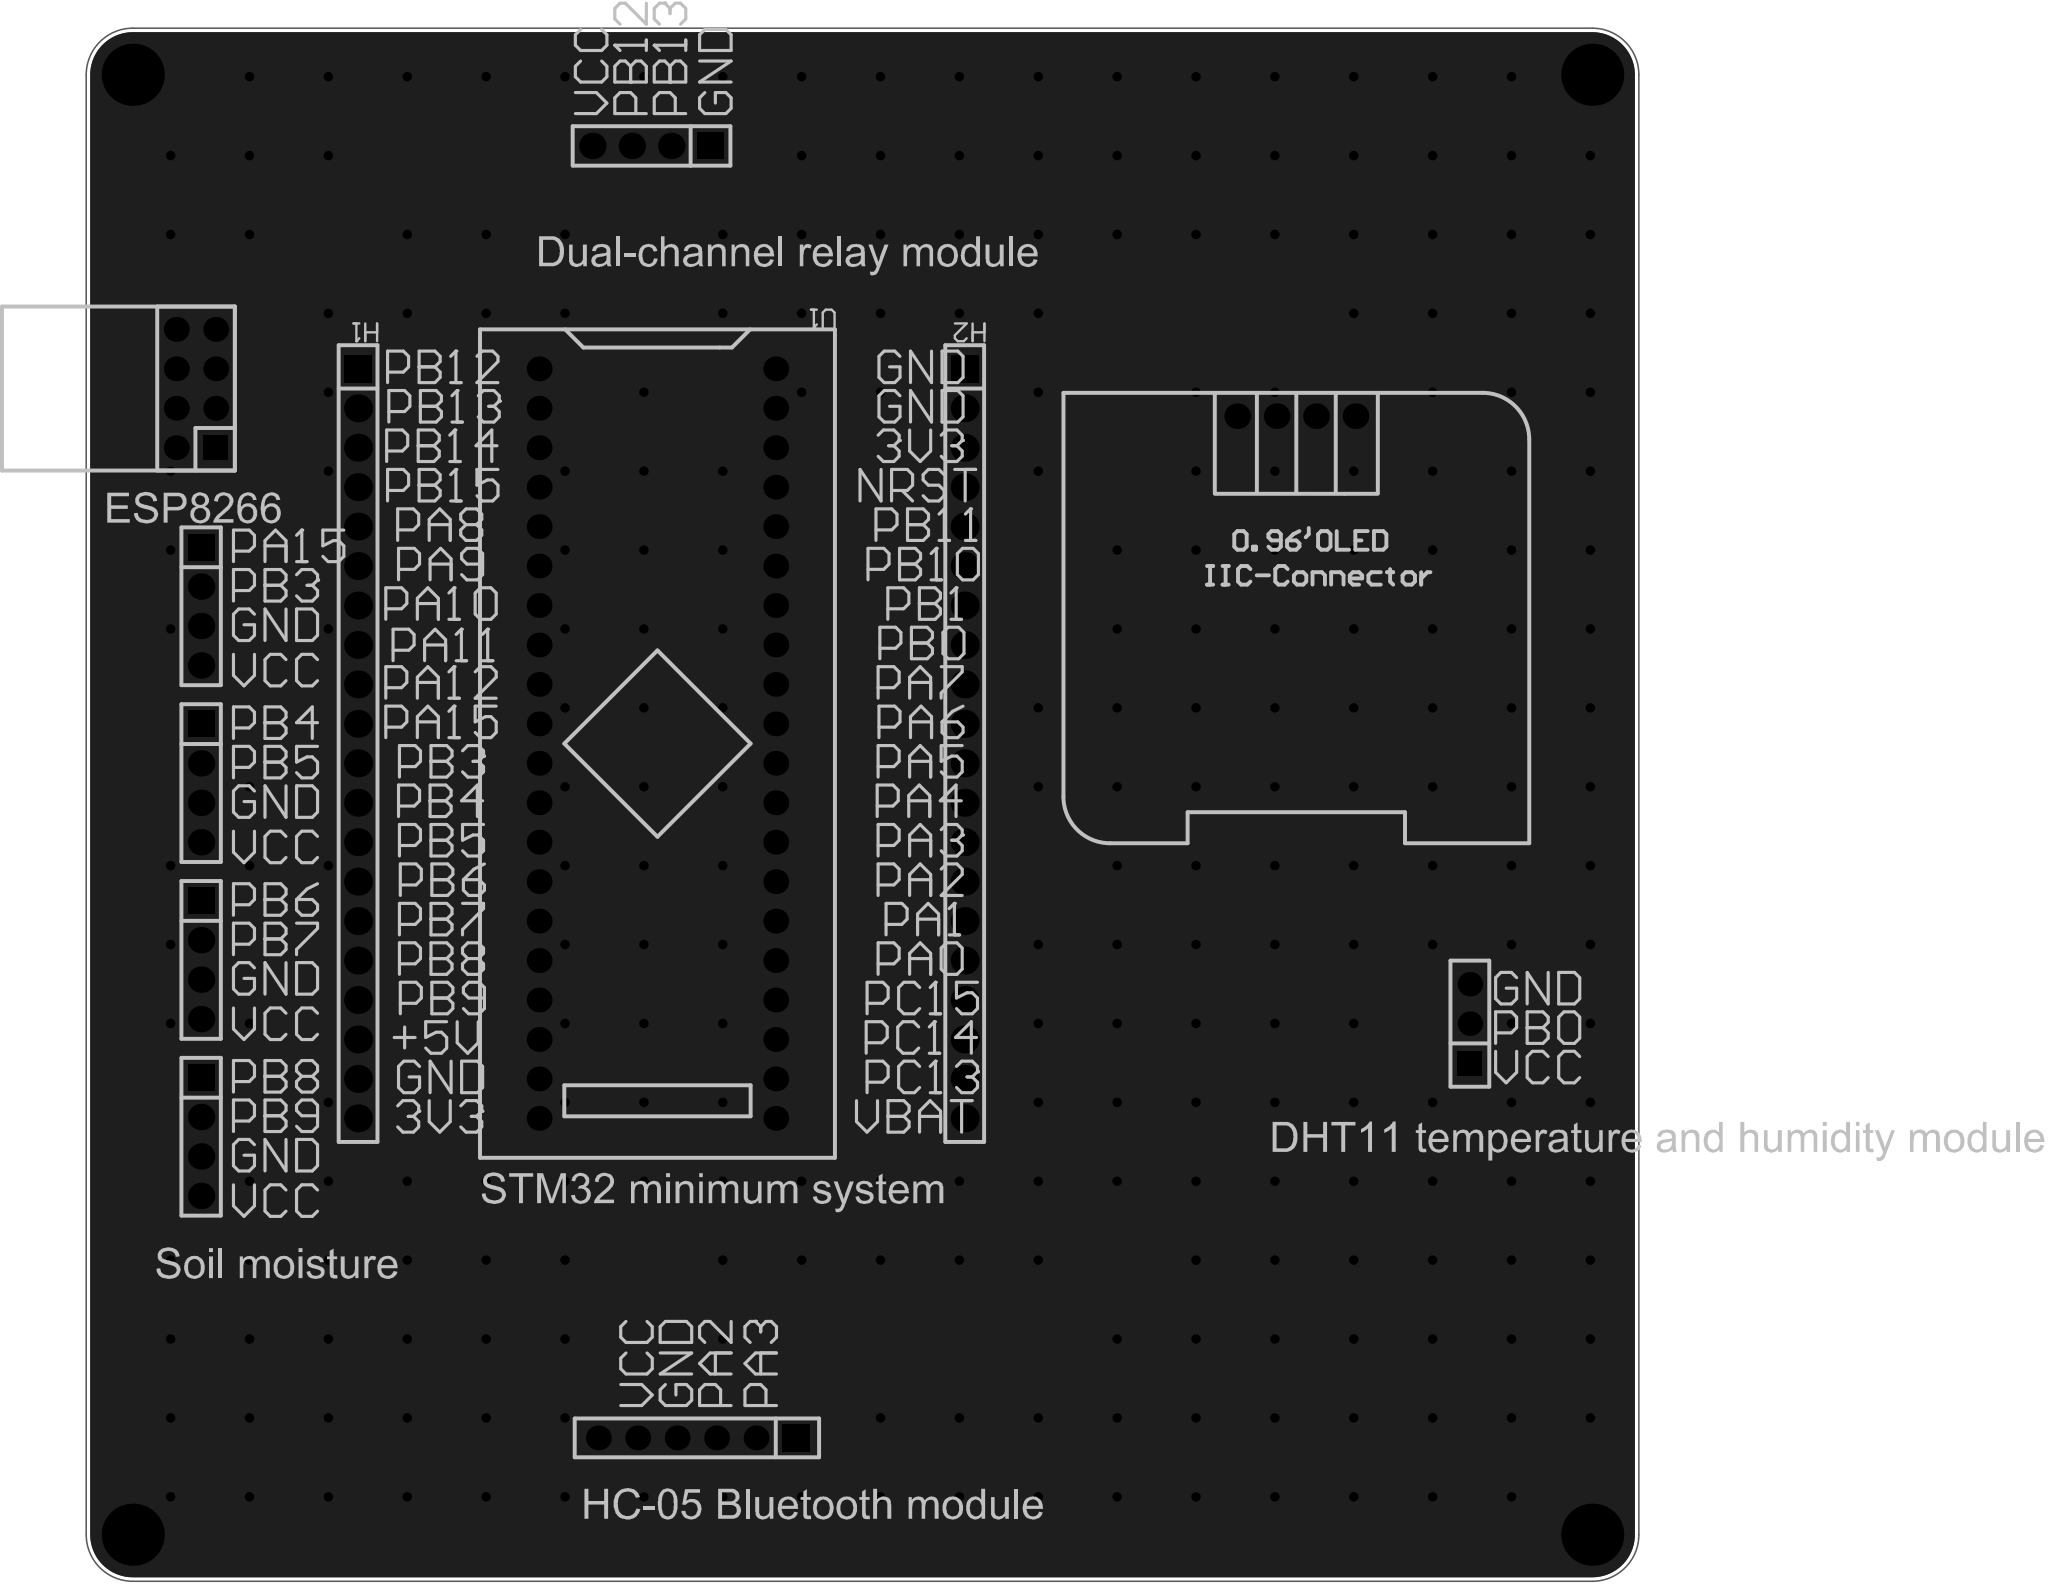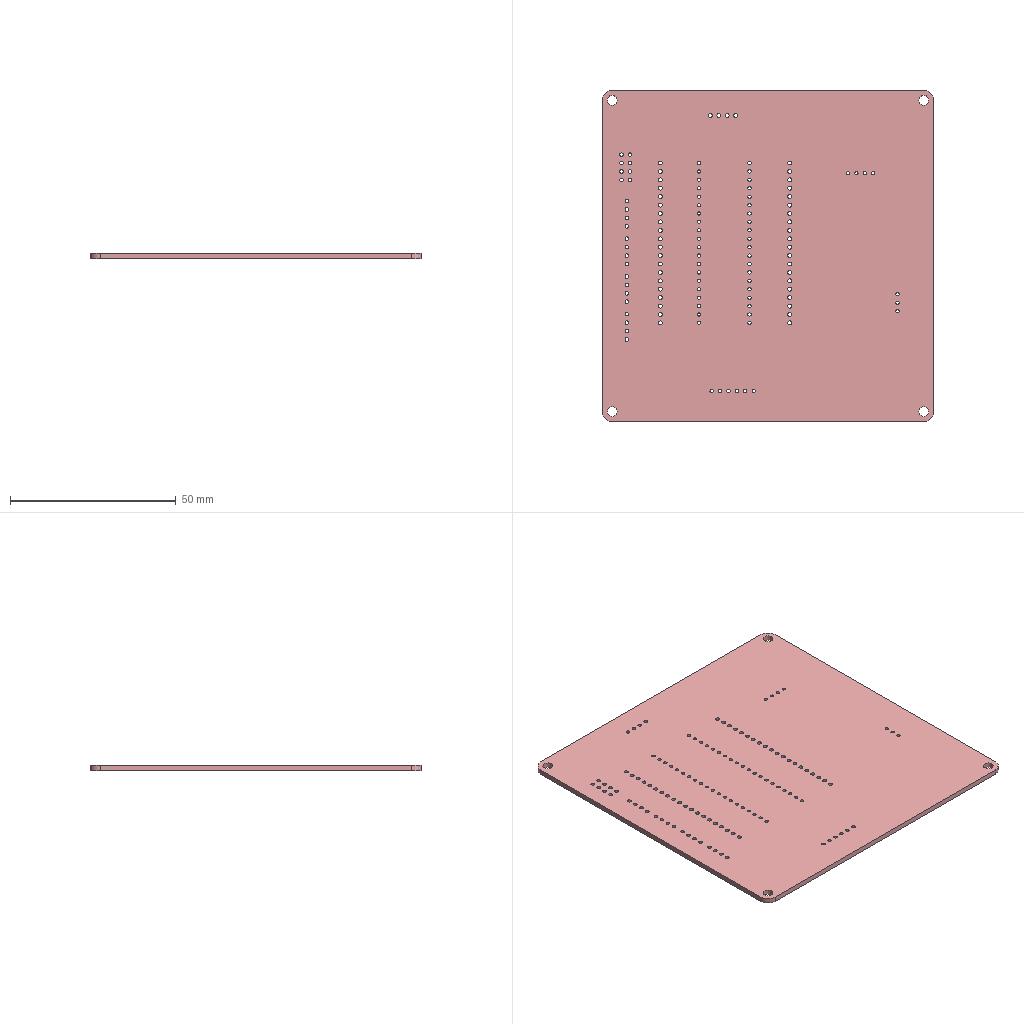Circuit board layout | Altium Designer | box 100 x 100 x 1.6 mm
Layer stack:
# Altium Designer layer stack of  (unit mm; dielectric type: 0 none, 1 core, 2 prepreg, 3 surface material)
index,name,kind,layer,copper_thickness_mm,dielectric_type,dielectric_thickness_mm,dielectric_material,dielectric_constant
0,Top Paste Mask Layer,other,,,,,,
1,Top Silkscreen Layer,other,,,,,,
2,Top Solder Mask Layer,dielectric,,,3,0.01,,3.3
3,Top Layer,copper,Top Layer,0.035,,,,
4,Dielectric1,dielectric,,,3,1.51,FR4,4.5
5,Bottom Layer,copper,Bottom Layer,0.035,,,,
6,Bottom Solder Mask Layer,dielectric,,,3,0.01,,3.3
7,Bottom Silkscreen Layer,other,,,,,,
8,Bottom Paste Mask Layer,other,,,,,,
# drill layer pairs: low layer,high layer
drill_pair,Top Layer,Bottom Layer
Part placement:
Designator,Comment,Layer,Footprint,Center-X(mm),Center-Y(mm),Rotation
U1,STM32F103C8T6-Card,TopLayer,CONN-TH_L53.3-W22.9_STM32F103C8T6-CARD,118.418,132.842,270
H22,,TopLayer,HDR-TH_6P-P2.54-V-F,120.958,88.138,180
H23,HDR2.54-LI-2x4P,TopLayer,HDR-TH_4P-P2.54-V-M,89.027,141.683,270
OLED1,,TopLayer,0.96OLED_4P,159.566,153.924,0
H24,HDR2.54-LI-2x4P,TopLayer,HDR-TH_4P-P2.54-V-M,89.027,118.912,270
H15,,TopLayer,HDR-TH_3P-P2.54-V-F,170.742,114.808,90
H16,,TopLayer,HDR-TH_8P-P2.54-V-F-R2-C4-S2.54-1,88.7,155.702,90
H1,,TopLayer,HDR-TH_20P-P2.54-V-F,99.135,132.842,270
H2,,TopLayer,HDR-TH_20P-P2.54-V-F,138.206,132.842,270
H25,HDR2.54-LI-2x4P,TopLayer,HDR-TH_4P-P2.54-V-M,89.027,130.298,270
H26,HDR2.54-LI-2x4P,TopLayer,HDR-TH_4P-P2.54-V-M,89.027,107.528,270
H20,HDR2.54-LI-2x4P,TopLayer,HDR-TH_4P-P2.54-V-M,118.037,171.323,180
Pad and via stacks:
# Altium Designer via and pad stacks of  (unit mm). Each distinct definition once, with the count of objects using it.
# via: kind,start_layer,end_layer,hole_mm,diameter_mm,mode(0 simple;1 top-mid-bottom;2 full stack),diameter_per_layer,count,example_net
# pad: kind,layer,hole_mm,hole_type(0 round;1 square;2 slot),plating,top_size,top_shape(1 round;2 rect;3 octagon;9 rounded rect),mid_size,bottom_size,mode,footprint,size_per_layer,count,example
pad,Multi-Layer,3,0,plated,4x4,1,4x4,4x4,0,,,4,1
pad,Multi-Layer,1,0,plated,1.6x1.6,1,1.6x1.6,1.6x1.6,0,CONN-TH_L53.3-W22.9_STM32F103C8T6-CARD,,40,U1.1
pad,Multi-Layer,1.02,0,plated,1.6x1.6,1,1.6x1.6,1.6x1.6,0,HDR-TH_6P-P2.54-V-F,,5,H22.6
pad,Multi-Layer,1.02,0,plated,1.8x1.8,2,1.8x1.8,1.8x1.8,0,HDR-TH_6P-P2.54-V-F,,1,H22.1
pad,Multi-Layer,1.1,0,plated,1.7x1.7,2,1.7x1.7,1.7x1.7,0,HDR-TH_4P-P2.54-V-M,,5,H23.1
pad,Multi-Layer,1.1,0,plated,1.7x1.7,1,1.7x1.7,1.7x1.7,0,HDR-TH_4P-P2.54-V-M,,15,H23.2
pad,Multi-Layer,1,0,plated,1.65x1.65,1,1.65x1.65,1.65x1.65,0,0.96OLED_4P,,4,OLED1.4
pad,Multi-Layer,1.02,0,plated,1.575x1.575,1,1.575x1.575,1.575x1.575,0,HDR-TH_3P-P2.54-V-F,,2,H15.3
pad,Multi-Layer,1.02,0,plated,1.575x1.575,2,1.575x1.575,1.575x1.575,0,HDR-TH_3P-P2.54-V-F,,1,H15.1
pad,Multi-Layer,1.1,0,plated,1.6x1.6,2,1.6x1.6,1.6x1.6,0,HDR-TH_8P-P2.54-V-F-R2-C4-S2.54-1,,1,H16.1
pad,Multi-Layer,1.1,0,plated,1.6x1.6,1,1.6x1.6,1.6x1.6,0,HDR-TH_8P-P2.54-V-F-R2-C4-S2.54-1,,7,H16.2
pad,Multi-Layer,1.2,0,plated,1.8x1.8,2,1.8x1.8,1.8x1.8,0,HDR-TH_20P-P2.54-V-F,,2,H1.1
pad,Multi-Layer,1.2,0,plated,1.8x1.8,1,1.8x1.8,1.8x1.8,0,HDR-TH_20P-P2.54-V-F,,38,H1.2
via,Top Layer,Bottom Layer,0.3048,0.61,0,,261,GND
Copper pours:
name,layer,net,type(0 solid;1 hatched;2 none)
Bottom Layer-GND,Bottom Layer,GND,0
Top Layer-GND,Top Layer,GND,0